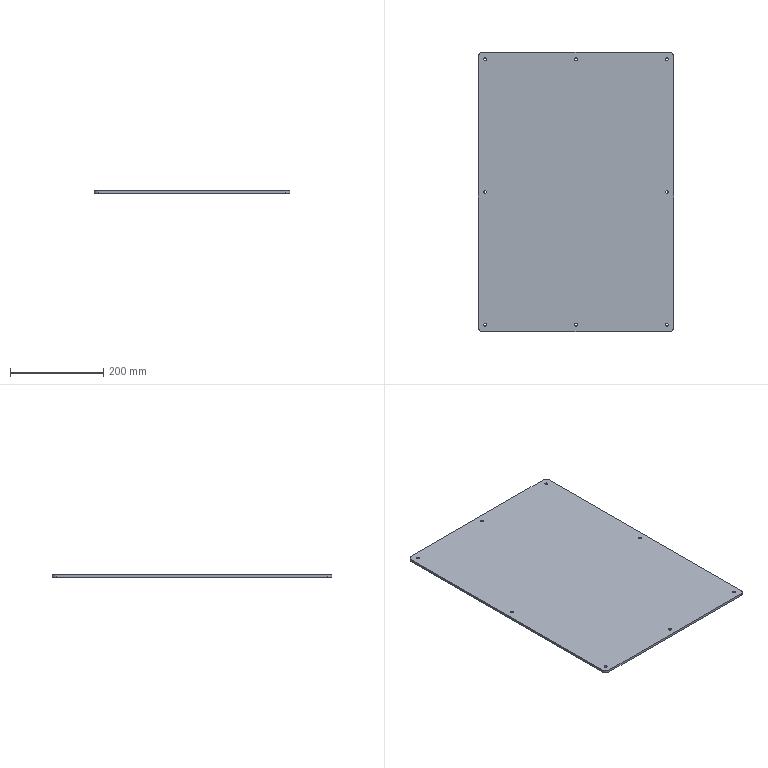Part | STEP file | PN_0012 | 1 solid | 26 faces | box 420 x 600 x 5 mm | volume 1258440 mm3 | cylinder 20 | plane 6 | commonest cylinder face diameters 6 x16 20 x4